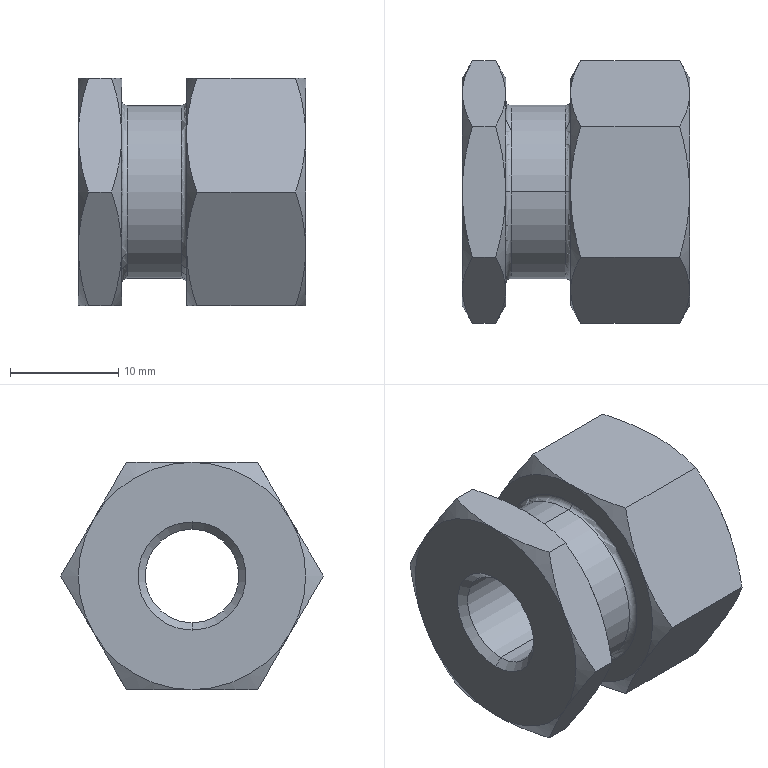Part | STEP file | 11-FJR10_1_25_6CW11_FJR10-1.25-6 | 1 solid | 52 faces | box 21 x 24.249 x 21 mm | volume 5654 mm3 | cone 28 | plane 16 | cylinder 4 | torus 4 | commonest cylinder face diameters 8.647 x2 16 x2